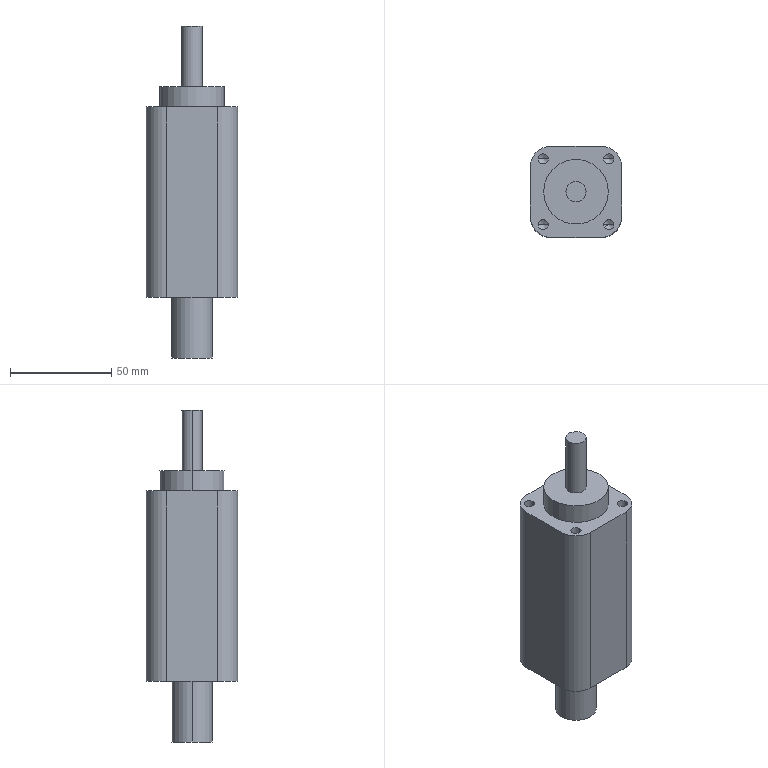Part | 1 solid | 35 faces | box 45 x 45 x 164 mm | volume 200887 mm3 | cylinder 18 | plane 9 | cone 8 | commonest cylinder face diameters 5 x8 20 x6 10 x2 32 x2
STEP:
#1=CARTESIAN_POINT('',(-10.,0.,-30.));
#2=VERTEX_POINT('',#1);
#3=CARTESIAN_POINT('',(10.,0.,-30.));
#4=VERTEX_POINT('',#3);
#5=CARTESIAN_POINT('',(0.,0.,-30.));
#6=DIRECTION('',(0.,0.,-1.));
#7=DIRECTION('',(-1.,0.,0.));
#8=AXIS2_PLACEMENT_3D('',#5,#6,#7);
#9=CIRCLE('',#8,10.);
#10=EDGE_CURVE('',#2,#4,#9,.T.);
#11=ORIENTED_EDGE('',*,*,#10,.F.);
#12=CARTESIAN_POINT('',(-10.,0.,0.));
#13=VERTEX_POINT('',#12);
#14=CARTESIAN_POINT('',(-10.,0.,-30.));
#15=DIRECTION('',(0.,0.,1.));
#16=VECTOR('',#15,1000.);
#17=LINE('',#14,#16);
#18=EDGE_CURVE('',#2,#13,#17,.T.);
#19=ORIENTED_EDGE('',*,*,#18,.T.);
#20=CARTESIAN_POINT('',(10.,0.,0.));
#21=VERTEX_POINT('',#20);
#22=CARTESIAN_POINT('',(0.,0.,0.));
#23=DIRECTION('',(0.,0.,-1.));
#24=DIRECTION('',(-1.,0.,0.));
#25=AXIS2_PLACEMENT_3D('',#22,#23,#24);
#26=CIRCLE('',#25,10.);
#27=EDGE_CURVE('',#13,#21,#26,.T.);
#28=ORIENTED_EDGE('',*,*,#27,.T.);
#29=CARTESIAN_POINT('',(10.,0.,-30.));
#30=DIRECTION('',(0.,0.,1.));
#31=VECTOR('',#30,1000.);
#32=LINE('',#29,#31);
#33=EDGE_CURVE('',#4,#21,#32,.T.);
#34=ORIENTED_EDGE('',*,*,#33,.F.);
#35=EDGE_LOOP('',(#11,#19,#28,#34));
#36=FACE_OUTER_BOUND('',#35,.T.);
#37=CARTESIAN_POINT('',(0.,0.,-30.));
#38=DIRECTION('',(0.,0.,1.));
#39=DIRECTION('',(1.,0.,0.));
#40=AXIS2_PLACEMENT_3D('',#37,#38,#39);
#41=CYLINDRICAL_SURFACE('',#40,10.);
#42=ADVANCED_FACE('',(#36),#41,.T.);
#43=CARTESIAN_POINT('',(5.,0.,134.));
#44=VERTEX_POINT('',#43);
#45=CARTESIAN_POINT('',(-5.,0.,134.));
#46=VERTEX_POINT('',#45);
#47=CARTESIAN_POINT('',(0.,0.,134.));
#48=DIRECTION('',(0.,0.,1.));
#49=DIRECTION('',(1.,0.,0.));
#50=AXIS2_PLACEMENT_3D('',#47,#48,#49);
#51=CIRCLE('',#50,5.);
#52=EDGE_CURVE('',#44,#46,#51,.T.);
#53=ORIENTED_EDGE('',*,*,#52,.F.);
#54=CARTESIAN_POINT('',(5.,0.,104.));
#55=VERTEX_POINT('',#54);
#56=CARTESIAN_POINT('',(5.,0.,134.));
#57=DIRECTION('',(0.,0.,-1.));
#58=VECTOR('',#57,1000.);
#59=LINE('',#56,#58);
#60=EDGE_CURVE('',#44,#55,#59,.T.);
#61=ORIENTED_EDGE('',*,*,#60,.T.);
#62=CARTESIAN_POINT('',(-5.,0.,104.));
#63=VERTEX_POINT('',#62);
#64=CARTESIAN_POINT('',(0.,0.,104.));
#65=DIRECTION('',(0.,0.,1.));
#66=DIRECTION('',(1.,0.,0.));
#67=AXIS2_PLACEMENT_3D('',#64,#65,#66);
#68=CIRCLE('',#67,5.);
#69=EDGE_CURVE('',#55,#63,#68,.T.);
#70=ORIENTED_EDGE('',*,*,#69,.T.);
#71=CARTESIAN_POINT('',(-5.,0.,134.));
#72=DIRECTION('',(0.,0.,-1.));
#73=VECTOR('',#72,1000.);
#74=LINE('',#71,#73);
#75=EDGE_CURVE('',#46,#63,#74,.T.);
#76=ORIENTED_EDGE('',*,*,#75,.F.);
#77=EDGE_LOOP('',(#53,#61,#70,#76));
#78=FACE_OUTER_BOUND('',#77,.T.);
#79=CARTESIAN_POINT('',(0.,0.,134.));
#80=DIRECTION('',(0.,0.,-1.));
#81=DIRECTION('',(-1.,0.,0.));
#82=AXIS2_PLACEMENT_3D('',#79,#80,#81);
#83=CYLINDRICAL_SURFACE('',#82,5.);
#84=ADVANCED_FACE('',(#78),#83,.T.);
#85=CARTESIAN_POINT('',(16.,0.,104.));
#86=VERTEX_POINT('',#85);
#87=CARTESIAN_POINT('',(-16.,0.,104.));
#88=VERTEX_POINT('',#87);
#89=CARTESIAN_POINT('',(0.,0.,104.));
#90=DIRECTION('',(0.,0.,1.));
#91=DIRECTION('',(1.,0.,0.));
#92=AXIS2_PLACEMENT_3D('',#89,#90,#91);
#93=CIRCLE('',#92,16.);
#94=EDGE_CURVE('',#86,#88,#93,.T.);
#95=ORIENTED_EDGE('',*,*,#94,.F.);
#96=CARTESIAN_POINT('',(16.,0.,94.));
#97=VERTEX_POINT('',#96);
#98=CARTESIAN_POINT('',(16.,0.,104.));
#99=DIRECTION('',(0.,0.,-1.));
#100=VECTOR('',#99,1000.);
#101=LINE('',#98,#100);
#102=EDGE_CURVE('',#86,#97,#101,.T.);
#103=ORIENTED_EDGE('',*,*,#102,.T.);
#104=CARTESIAN_POINT('',(-16.,0.,94.));
#105=VERTEX_POINT('',#104);
#106=CARTESIAN_POINT('',(0.,0.,94.));
#107=DIRECTION('',(0.,0.,1.));
#108=DIRECTION('',(-1.,0.,0.));
#109=AXIS2_PLACEMENT_3D('',#106,#107,#108);
#110=CIRCLE('',#109,16.);
#111=EDGE_CURVE('',#97,#105,#110,.T.);
#112=ORIENTED_EDGE('',*,*,#111,.T.);
#113=CARTESIAN_POINT('',(-16.,0.,104.));
#114=DIRECTION('',(0.,0.,-1.));
#115=VECTOR('',#114,1000.);
#116=LINE('',#113,#115);
#117=EDGE_CURVE('',#88,#105,#116,.T.);
#118=ORIENTED_EDGE('',*,*,#117,.F.);
#119=EDGE_LOOP('',(#95,#103,#112,#118));
#120=FACE_OUTER_BOUND('',#119,.T.);
#121=CARTESIAN_POINT('',(0.,0.,104.));
#122=DIRECTION('',(0.,0.,-1.));
#123=DIRECTION('',(-1.,0.,0.));
#124=AXIS2_PLACEMENT_3D('',#121,#122,#123);
#125=CYLINDRICAL_SURFACE('',#124,16.);
#126=ADVANCED_FACE('',(#120),#125,.T.);
#127=CARTESIAN_POINT('',(-18.75,16.25,79.));
#128=VERTEX_POINT('',#127);
#129=CARTESIAN_POINT('',(-13.75,16.25,79.));
#130=VERTEX_POINT('',#129);
#131=CARTESIAN_POINT('',(-16.25,16.25,79.));
#132=DIRECTION('',(0.,0.,1.));
#133=DIRECTION('',(1.,0.,0.));
#134=AXIS2_PLACEMENT_3D('',#131,#132,#133);
#135=CIRCLE('',#134,2.5);
#136=EDGE_CURVE('',#128,#130,#135,.T.);
#137=ORIENTED_EDGE('',*,*,#136,.F.);
#138=CARTESIAN_POINT('',(-18.75,16.25,94.));
#139=VERTEX_POINT('',#138);
#140=CARTESIAN_POINT('',(-18.75,16.25,94.));
#141=DIRECTION('',(0.,0.,1.));
#142=VECTOR('',#141,1000.);
#143=LINE('',#140,#142);
#144=EDGE_CURVE('',#128,#139,#143,.T.);
#145=ORIENTED_EDGE('',*,*,#144,.T.);
#146=CARTESIAN_POINT('',(-13.75,16.25,94.));
#147=VERTEX_POINT('',#146);
#148=CARTESIAN_POINT('',(-16.25,16.25,94.));
#149=DIRECTION('',(0.,0.,1.));
#150=DIRECTION('',(1.,0.,0.));
#151=AXIS2_PLACEMENT_3D('',#148,#149,#150);
#152=CIRCLE('',#151,2.5);
#153=EDGE_CURVE('',#139,#147,#152,.T.);
#154=ORIENTED_EDGE('',*,*,#153,.T.);
#155=CARTESIAN_POINT('',(-13.75,16.25,94.));
#156=DIRECTION('',(0.,0.,1.));
#157=VECTOR('',#156,1000.);
#158=LINE('',#155,#157);
#159=EDGE_CURVE('',#130,#147,#158,.T.);
#160=ORIENTED_EDGE('',*,*,#159,.F.);
#161=EDGE_LOOP('',(#137,#145,#154,#160));
#162=FACE_OUTER_BOUND('',#161,.T.);
#163=CARTESIAN_POINT('',(-16.25,16.25,94.));
#164=DIRECTION('',(0.,0.,1.));
#165=DIRECTION('',(1.,0.,0.));
#166=AXIS2_PLACEMENT_3D('',#163,#164,#165);
#167=CYLINDRICAL_SURFACE('',#166,2.5);
#168=ADVANCED_FACE('',(#162),#167,.F.);
#169=CARTESIAN_POINT('',(-16.25,16.25,77.498));
#170=VERTEX_POINT('',#169);
#171=CARTESIAN_POINT('',(-13.75,16.25,79.));
#172=DIRECTION('',(0.8572,0.,0.515));
#173=VECTOR('',#172,1000.);
#174=LINE('',#171,#173);
#175=EDGE_CURVE('',#170,#130,#174,.T.);
#176=ORIENTED_EDGE('',*,*,#175,.F.);
#177=CARTESIAN_POINT('',(-18.75,16.25,79.));
#178=DIRECTION('',(-0.8572,0.,0.515));
#179=VECTOR('',#178,1000.);
#180=LINE('',#177,#179);
#181=EDGE_CURVE('',#170,#128,#180,.T.);
#182=ORIENTED_EDGE('',*,*,#181,.T.);
#183=ORIENTED_EDGE('',*,*,#136,.T.);
#184=EDGE_LOOP('',(#176,#182,#183));
#185=FACE_OUTER_BOUND('',#184,.T.);
#186=CARTESIAN_POINT('',(-16.25,16.25,79.));
#187=DIRECTION('',(0.,0.,1.));
#188=DIRECTION('',(1.,0.,0.));
#189=AXIS2_PLACEMENT_3D('',#186,#187,#188);
#190=CONICAL_SURFACE('',#189,2.5,1.03);
#191=ADVANCED_FACE('',(#185),#190,.F.);
#192=CARTESIAN_POINT('',(13.75,16.25,79.));
#193=VERTEX_POINT('',#192);
#194=CARTESIAN_POINT('',(18.75,16.25,79.));
#195=VERTEX_POINT('',#194);
#196=CARTESIAN_POINT('',(16.25,16.25,79.));
#197=DIRECTION('',(0.,0.,1.));
#198=DIRECTION('',(1.,0.,0.));
#199=AXIS2_PLACEMENT_3D('',#196,#197,#198);
#200=CIRCLE('',#199,2.5);
#201=EDGE_CURVE('',#193,#195,#200,.T.);
#202=ORIENTED_EDGE('',*,*,#201,.F.);
#203=CARTESIAN_POINT('',(13.75,16.25,94.));
#204=VERTEX_POINT('',#203);
#205=CARTESIAN_POINT('',(13.75,16.25,94.));
#206=DIRECTION('',(0.,0.,1.));
#207=VECTOR('',#206,1000.);
#208=LINE('',#205,#207);
#209=EDGE_CURVE('',#193,#204,#208,.T.);
#210=ORIENTED_EDGE('',*,*,#209,.T.);
#211=CARTESIAN_POINT('',(18.75,16.25,94.));
#212=VERTEX_POINT('',#211);
#213=CARTESIAN_POINT('',(16.25,16.25,94.));
#214=DIRECTION('',(0.,0.,1.));
#215=DIRECTION('',(1.,0.,0.));
#216=AXIS2_PLACEMENT_3D('',#213,#214,#215);
#217=CIRCLE('',#216,2.5);
#218=EDGE_CURVE('',#204,#212,#217,.T.);
#219=ORIENTED_EDGE('',*,*,#218,.T.);
#220=CARTESIAN_POINT('',(18.75,16.25,94.));
#221=DIRECTION('',(0.,0.,1.));
#222=VECTOR('',#221,1000.);
#223=LINE('',#220,#222);
#224=EDGE_CURVE('',#195,#212,#223,.T.);
#225=ORIENTED_EDGE('',*,*,#224,.F.);
#226=EDGE_LOOP('',(#202,#210,#219,#225));
#227=FACE_OUTER_BOUND('',#226,.T.);
#228=CARTESIAN_POINT('',(16.25,16.25,94.));
#229=DIRECTION('',(0.,0.,1.));
#230=DIRECTION('',(1.,0.,0.));
#231=AXIS2_PLACEMENT_3D('',#228,#229,#230);
#232=CYLINDRICAL_SURFACE('',#231,2.5);
#233=ADVANCED_FACE('',(#227),#232,.F.);
#234=CARTESIAN_POINT('',(16.25,16.25,77.498));
#235=VERTEX_POINT('',#234);
#236=CARTESIAN_POINT('',(18.75,16.25,79.));
#237=DIRECTION('',(0.8572,0.,0.515));
#238=VECTOR('',#237,1000.);
#239=LINE('',#236,#238);
#240=EDGE_CURVE('',#235,#195,#239,.T.);
#241=ORIENTED_EDGE('',*,*,#240,.F.);
#242=CARTESIAN_POINT('',(13.75,16.25,79.));
#243=DIRECTION('',(-0.8572,0.,0.515));
#244=VECTOR('',#243,1000.);
#245=LINE('',#242,#244);
#246=EDGE_CURVE('',#235,#193,#245,.T.);
#247=ORIENTED_EDGE('',*,*,#246,.T.);
#248=ORIENTED_EDGE('',*,*,#201,.T.);
#249=EDGE_LOOP('',(#241,#247,#248));
#250=FACE_OUTER_BOUND('',#249,.T.);
#251=CARTESIAN_POINT('',(16.25,16.25,79.));
#252=DIRECTION('',(0.,0.,1.));
#253=DIRECTION('',(1.,0.,0.));
#254=AXIS2_PLACEMENT_3D('',#251,#252,#253);
#255=CONICAL_SURFACE('',#254,2.5,1.03);
#256=ADVANCED_FACE('',(#250),#255,.F.);
#257=CARTESIAN_POINT('',(-18.75,-16.25,79.));
#258=VERTEX_POINT('',#257);
#259=CARTESIAN_POINT('',(-13.75,-16.25,79.));
#260=VERTEX_POINT('',#259);
#261=CARTESIAN_POINT('',(-16.25,-16.25,79.));
#262=DIRECTION('',(0.,0.,1.));
#263=DIRECTION('',(1.,0.,0.));
#264=AXIS2_PLACEMENT_3D('',#261,#262,#263);
#265=CIRCLE('',#264,2.5);
#266=EDGE_CURVE('',#258,#260,#265,.T.);
#267=ORIENTED_EDGE('',*,*,#266,.F.);
#268=CARTESIAN_POINT('',(-18.75,-16.25,94.));
#269=VERTEX_POINT('',#268);
#270=CARTESIAN_POINT('',(-18.75,-16.25,94.));
#271=DIRECTION('',(0.,0.,1.));
#272=VECTOR('',#271,1000.);
#273=LINE('',#270,#272);
#274=EDGE_CURVE('',#258,#269,#273,.T.);
#275=ORIENTED_EDGE('',*,*,#274,.T.);
#276=CARTESIAN_POINT('',(-13.75,-16.25,94.));
#277=VERTEX_POINT('',#276);
#278=CARTESIAN_POINT('',(-16.25,-16.25,94.));
#279=DIRECTION('',(0.,0.,1.));
#280=DIRECTION('',(1.,0.,0.));
#281=AXIS2_PLACEMENT_3D('',#278,#279,#280);
#282=CIRCLE('',#281,2.5);
#283=EDGE_CURVE('',#269,#277,#282,.T.);
#284=ORIENTED_EDGE('',*,*,#283,.T.);
#285=CARTESIAN_POINT('',(-13.75,-16.25,94.));
#286=DIRECTION('',(0.,0.,1.));
#287=VECTOR('',#286,1000.);
#288=LINE('',#285,#287);
#289=EDGE_CURVE('',#260,#277,#288,.T.);
#290=ORIENTED_EDGE('',*,*,#289,.F.);
#291=EDGE_LOOP('',(#267,#275,#284,#290));
#292=FACE_OUTER_BOUND('',#291,.T.);
#293=CARTESIAN_POINT('',(-16.25,-16.25,94.));
#294=DIRECTION('',(0.,0.,1.));
#295=DIRECTION('',(1.,0.,0.));
#296=AXIS2_PLACEMENT_3D('',#293,#294,#295);
#297=CYLINDRICAL_SURFACE('',#296,2.5);
#298=ADVANCED_FACE('',(#292),#297,.F.);
#299=CARTESIAN_POINT('',(-16.25,-16.25,77.498));
#300=VERTEX_POINT('',#299);
#301=CARTESIAN_POINT('',(-13.75,-16.25,79.));
#302=DIRECTION('',(0.8572,0.,0.515));
#303=VECTOR('',#302,1000.);
#304=LINE('',#301,#303);
#305=EDGE_CURVE('',#300,#260,#304,.T.);
#306=ORIENTED_EDGE('',*,*,#305,.F.);
#307=CARTESIAN_POINT('',(-18.75,-16.25,79.));
#308=DIRECTION('',(-0.8572,0.,0.515));
#309=VECTOR('',#308,1000.);
#310=LINE('',#307,#309);
#311=EDGE_CURVE('',#300,#258,#310,.T.);
#312=ORIENTED_EDGE('',*,*,#311,.T.);
#313=ORIENTED_EDGE('',*,*,#266,.T.);
#314=EDGE_LOOP('',(#306,#312,#313));
#315=FACE_OUTER_BOUND('',#314,.T.);
#316=CARTESIAN_POINT('',(-16.25,-16.25,79.));
#317=DIRECTION('',(0.,0.,1.));
#318=DIRECTION('',(1.,0.,0.));
#319=AXIS2_PLACEMENT_3D('',#316,#317,#318);
#320=CONICAL_SURFACE('',#319,2.5,1.03);
#321=ADVANCED_FACE('',(#315),#320,.F.);
#322=CARTESIAN_POINT('',(13.75,-16.25,79.));
#323=VERTEX_POINT('',#322);
#324=CARTESIAN_POINT('',(18.75,-16.25,79.));
#325=VERTEX_POINT('',#324);
#326=CARTESIAN_POINT('',(16.25,-16.25,79.));
#327=DIRECTION('',(0.,0.,1.));
#328=DIRECTION('',(1.,0.,0.));
#329=AXIS2_PLACEMENT_3D('',#326,#327,#328);
#330=CIRCLE('',#329,2.5);
#331=EDGE_CURVE('',#323,#325,#330,.T.);
#332=ORIENTED_EDGE('',*,*,#331,.F.);
#333=CARTESIAN_POINT('',(13.75,-16.25,94.));
#334=VERTEX_POINT('',#333);
#335=CARTESIAN_POINT('',(13.75,-16.25,94.));
#336=DIRECTION('',(0.,0.,1.));
#337=VECTOR('',#336,1000.);
#338=LINE('',#335,#337);
#339=EDGE_CURVE('',#323,#334,#338,.T.);
#340=ORIENTED_EDGE('',*,*,#339,.T.);
#341=CARTESIAN_POINT('',(18.75,-16.25,94.));
#342=VERTEX_POINT('',#341);
#343=CARTESIAN_POINT('',(16.25,-16.25,94.));
#344=DIRECTION('',(0.,0.,1.));
#345=DIRECTION('',(1.,0.,0.));
#346=AXIS2_PLACEMENT_3D('',#343,#344,#345);
#347=CIRCLE('',#346,2.5);
#348=EDGE_CURVE('',#334,#342,#347,.T.);
#349=ORIENTED_EDGE('',*,*,#348,.T.);
#350=CARTESIAN_POINT('',(18.75,-16.25,94.));
#351=DIRECTION('',(0.,0.,1.));
#352=VECTOR('',#351,1000.);
#353=LINE('',#350,#352);
#354=EDGE_CURVE('',#325,#342,#353,.T.);
#355=ORIENTED_EDGE('',*,*,#354,.F.);
#356=EDGE_LOOP('',(#332,#340,#349,#355));
#357=FACE_OUTER_BOUND('',#356,.T.);
#358=CARTESIAN_POINT('',(16.25,-16.25,94.));
#359=DIRECTION('',(0.,0.,1.));
#360=DIRECTION('',(1.,0.,0.));
#361=AXIS2_PLACEMENT_3D('',#358,#359,#360);
#362=CYLINDRICAL_SURFACE('',#361,2.5);
#363=ADVANCED_FACE('',(#357),#362,.F.);
#364=CARTESIAN_POINT('',(16.25,-16.25,77.498));
#365=VERTEX_POINT('',#364);
#366=CARTESIAN_POINT('',(18.75,-16.25,79.));
#367=DIRECTION('',(0.8572,0.,0.515));
#368=VECTOR('',#367,1000.);
#369=LINE('',#366,#368);
#370=EDGE_CURVE('',#365,#325,#369,.T.);
#371=ORIENTED_EDGE('',*,*,#370,.F.);
#372=CARTESIAN_POINT('',(13.75,-16.25,79.));
#373=DIRECTION('',(-0.8572,0.,0.515));
#374=VECTOR('',#373,1000.);
#375=LINE('',#372,#374);
#376=EDGE_CURVE('',#365,#323,#375,.T.);
#377=ORIENTED_EDGE('',*,*,#376,.T.);
#378=ORIENTED_EDGE('',*,*,#331,.T.);
#379=EDGE_LOOP('',(#371,#377,#378));
#380=FACE_OUTER_BOUND('',#379,.T.);
#381=CARTESIAN_POINT('',(16.25,-16.25,79.));
#382=DIRECTION('',(0.,0.,1.));
#383=DIRECTION('',(1.,0.,0.));
#384=AXIS2_PLACEMENT_3D('',#381,#382,#383);
#385=CONICAL_SURFACE('',#384,2.5,1.03);
#386=ADVANCED_FACE('',(#380),#385,.F.);
#387=CARTESIAN_POINT('',(-12.5,-22.5,0.));
#388=VERTEX_POINT('',#387);
#389=CARTESIAN_POINT('',(12.5,-22.5,0.));
#390=VERTEX_POINT('',#389);
#391=CARTESIAN_POINT('',(-22.5,-22.5,0.));
#392=DIRECTION('',(1.,0.,0.));
#393=VECTOR('',#392,1000.);
#394=LINE('',#391,#393);
#395=EDGE_CURVE('',#388,#390,#394,.T.);
#396=ORIENTED_EDGE('',*,*,#395,.F.);
#397=CARTESIAN_POINT('',(-22.5,-12.5,0.));
#398=VERTEX_POINT('',#397);
#399=CARTESIAN_POINT('',(-12.5,-12.5,0.));
#400=DIRECTION('',(0.,0.,-1.));
#401=DIRECTION('',(-1.,0.,0.));
#402=AXIS2_PLACEMENT_3D('',#399,#400,#401);
#403=CIRCLE('',#402,10.);
#404=EDGE_CURVE('',#388,#398,#403,.T.);
#405=ORIENTED_EDGE('',*,*,#404,.T.);
#406=CARTESIAN_POINT('',(-22.5,12.5,0.));
#407=VERTEX_POINT('',#406);
#408=CARTESIAN_POINT('',(-22.5,-22.5,0.));
#409=DIRECTION('',(0.,-1.,0.));
#410=VECTOR('',#409,1000.);
#411=LINE('',#408,#410);
#412=EDGE_CURVE('',#407,#398,#411,.T.);
#413=ORIENTED_EDGE('',*,*,#412,.F.);
#414=CARTESIAN_POINT('',(-12.5,22.5,0.));
#415=VERTEX_POINT('',#414);
#416=CARTESIAN_POINT('',(-12.5,12.5,0.));
#417=DIRECTION('',(0.,0.,-1.));
#418=DIRECTION('',(-1.,0.,0.));
#419=AXIS2_PLACEMENT_3D('',#416,#417,#418);
#420=CIRCLE('',#419,10.);
#421=EDGE_CURVE('',#407,#415,#420,.T.);
#422=ORIENTED_EDGE('',*,*,#421,.T.);
#423=CARTESIAN_POINT('',(12.5,22.5,0.));
#424=VERTEX_POINT('',#423);
#425=CARTESIAN_POINT('',(-22.5,22.5,0.));
#426=DIRECTION('',(-1.,0.,0.));
#427=VECTOR('',#426,1000.);
#428=LINE('',#425,#427);
#429=EDGE_CURVE('',#424,#415,#428,.T.);
#430=ORIENTED_EDGE('',*,*,#429,.F.);
#431=CARTESIAN_POINT('',(22.5,12.5,0.));
#432=VERTEX_POINT('',#431);
#433=CARTESIAN_POINT('',(12.5,12.5,0.));
#434=DIRECTION('',(0.,0.,-1.));
#435=DIRECTION('',(-1.,0.,0.));
#436=AXIS2_PLACEMENT_3D('',#433,#434,#435);
#437=CIRCLE('',#436,10.);
#438=EDGE_CURVE('',#424,#432,#437,.T.);
#439=ORIENTED_EDGE('',*,*,#438,.T.);
#440=CARTESIAN_POINT('',(22.5,-12.5,0.));
#441=VERTEX_POINT('',#440);
#442=CARTESIAN_POINT('',(22.5,-22.5,0.));
#443=DIRECTION('',(0.,1.,0.));
#444=VECTOR('',#443,1000.);
#445=LINE('',#442,#444);
#446=EDGE_CURVE('',#441,#432,#445,.T.);
#447=ORIENTED_EDGE('',*,*,#446,.F.);
#448=CARTESIAN_POINT('',(12.5,-12.5,0.));
#449=DIRECTION('',(0.,0.,-1.));
#450=DIRECTION('',(-1.,0.,0.));
#451=AXIS2_PLACEMENT_3D('',#448,#449,#450);
#452=CIRCLE('',#451,10.);
#453=EDGE_CURVE('',#441,#390,#452,.T.);
#454=ORIENTED_EDGE('',*,*,#453,.T.);
#455=EDGE_LOOP('',(#396,#405,#413,#422,#430,#439,#447,#454));
#456=FACE_OUTER_BOUND('',#455,.T.);
#457=CARTESIAN_POINT('',(0.,0.,0.));
#458=DIRECTION('',(0.,0.,-1.));
#459=DIRECTION('',(-1.,0.,0.));
#460=AXIS2_PLACEMENT_3D('',#457,#458,#459);
#461=CIRCLE('',#460,10.);
#462=EDGE_CURVE('',#21,#13,#461,.T.);
#463=ORIENTED_EDGE('',*,*,#462,.F.);
#464=ORIENTED_EDGE('',*,*,#27,.F.);
#465=EDGE_LOOP('',(#463,#464));
#466=FACE_BOUND('',#465,.T.);
#467=CARTESIAN_POINT('',(0.,0.,0.));
#468=DIRECTION('',(0.,0.,-1.));
#469=DIRECTION('',(-1.,0.,0.));
#470=AXIS2_PLACEMENT_3D('',#467,#468,#469);
#471=PLANE('',#470);
#472=ADVANCED_FACE('',(#456,#466),#471,.T.);
#473=CARTESIAN_POINT('',(0.,0.,104.));
#474=DIRECTION('',(0.,0.,1.));
#475=DIRECTION('',(1.,0.,0.));
#476=AXIS2_PLACEMENT_3D('',#473,#474,#475);
#477=CIRCLE('',#476,16.);
#478=EDGE_CURVE('',#88,#86,#477,.T.);
#479=ORIENTED_EDGE('',*,*,#478,.T.);
#480=ORIENTED_EDGE('',*,*,#94,.T.);
#481=EDGE_LOOP('',(#479,#480));
#482=FACE_OUTER_BOUND('',#481,.T.);
#483=CARTESIAN_POINT('',(0.,0.,104.));
#484=DIRECTION('',(0.,0.,1.));
#485=DIRECTION('',(1.,0.,0.));
#486=AXIS2_PLACEMENT_3D('',#483,#484,#485);
#487=CIRCLE('',#486,5.);
#488=EDGE_CURVE('',#63,#55,#487,.T.);
#489=ORIENTED_EDGE('',*,*,#488,.F.);
#490=ORIENTED_EDGE('',*,*,#69,.F.);
#491=EDGE_LOOP('',(#489,#490));
#492=FACE_BOUND('',#491,.T.);
#493=CARTESIAN_POINT('',(0.,0.,104.));
#494=DIRECTION('',(0.,0.,1.));
#495=DIRECTION('',(1.,0.,0.));
#496=AXIS2_PLACEMENT_3D('',#493,#494,#495);
#497=PLANE('',#496);
#498=ADVANCED_FACE('',(#482,#492),#497,.T.);
#499=CARTESIAN_POINT('',(-22.5,12.5,94.));
#500=VERTEX_POINT('',#499);
#501=CARTESIAN_POINT('',(-22.5,-12.5,94.));
#502=VERTEX_POINT('',#501);
#503=CARTESIAN_POINT('',(-22.5,-22.5,94.));
#504=DIRECTION('',(0.,-1.,0.));
#505=VECTOR('',#504,1000.);
#506=LINE('',#503,#505);
#507=EDGE_CURVE('',#500,#502,#506,.T.);
#508=ORIENTED_EDGE('',*,*,#507,.T.);
#509=CARTESIAN_POINT('',(-12.5,-22.5,94.));
#510=VERTEX_POINT('',#509);
#511=CARTESIAN_POINT('',(-12.5,-12.5,94.));
#512=DIRECTION('',(0.,0.,1.));
#513=DIRECTION('',(-1.,0.,0.));
#514=AXIS2_PLACEMENT_3D('',#511,#512,#513);
#515=CIRCLE('',#514,10.);
#516=EDGE_CURVE('',#502,#510,#515,.T.);
#517=ORIENTED_EDGE('',*,*,#516,.T.);
#518=CARTESIAN_POINT('',(12.5,-22.5,94.));
#519=VERTEX_POINT('',#518);
#520=CARTESIAN_POINT('',(-22.5,-22.5,94.));
#521=DIRECTION('',(1.,0.,0.));
#522=VECTOR('',#521,1000.);
#523=LINE('',#520,#522);
#524=EDGE_CURVE('',#510,#519,#523,.T.);
#525=ORIENTED_EDGE('',*,*,#524,.T.);
#526=CARTESIAN_POINT('',(22.5,-12.5,94.));
#527=VERTEX_POINT('',#526);
#528=CARTESIAN_POINT('',(12.5,-12.5,94.));
#529=DIRECTION('',(0.,0.,1.));
#530=DIRECTION('',(-1.,0.,0.));
#531=AXIS2_PLACEMENT_3D('',#528,#529,#530);
#532=CIRCLE('',#531,10.);
#533=EDGE_CURVE('',#519,#527,#532,.T.);
#534=ORIENTED_EDGE('',*,*,#533,.T.);
#535=CARTESIAN_POINT('',(22.5,12.5,94.));
#536=VERTEX_POINT('',#535);
#537=CARTESIAN_POINT('',(22.5,-22.5,94.));
#538=DIRECTION('',(0.,1.,0.));
#539=VECTOR('',#538,1000.);
#540=LINE('',#537,#539);
#541=EDGE_CURVE('',#527,#536,#540,.T.);
#542=ORIENTED_EDGE('',*,*,#541,.T.);
#543=CARTESIAN_POINT('',(12.5,22.5,94.));
#544=VERTEX_POINT('',#543);
#545=CARTESIAN_POINT('',(12.5,12.5,94.));
#546=DIRECTION('',(0.,0.,1.));
#547=DIRECTION('',(-1.,0.,0.));
#548=AXIS2_PLACEMENT_3D('',#545,#546,#547);
#549=CIRCLE('',#548,10.);
#550=EDGE_CURVE('',#536,#544,#549,.T.);
#551=ORIENTED_EDGE('',*,*,#550,.T.);
#552=CARTESIAN_POINT('',(-12.5,22.5,94.));
#553=VERTEX_POINT('',#552);
#554=CARTESIAN_POINT('',(-22.5,22.5,94.));
#555=DIRECTION('',(-1.,0.,0.));
#556=VECTOR('',#555,1000.);
#557=LINE('',#554,#556);
#558=EDGE_CURVE('',#544,#553,#557,.T.);
#559=ORIENTED_EDGE('',*,*,#558,.T.);
#560=CARTESIAN_POINT('',(-12.5,12.5,94.));
#561=DIRECTION('',(0.,0.,1.));
#562=DIRECTION('',(-1.,0.,0.));
#563=AXIS2_PLACEMENT_3D('',#560,#561,#562);
#564=CIRCLE('',#563,10.);
#565=EDGE_CURVE('',#553,#500,#564,.T.);
#566=ORIENTED_EDGE('',*,*,#565,.T.);
#567=EDGE_LOOP('',(#508,#517,#525,#534,#542,#551,#559,#566));
#568=FACE_OUTER_BOUND('',#567,.T.);
#569=CARTESIAN_POINT('',(16.25,-16.25,94.));
#570=DIRECTION('',(0.,0.,1.));
#571=DIRECTION('',(1.,0.,0.));
#572=AXIS2_PLACEMENT_3D('',#569,#570,#571);
#573=CIRCLE('',#572,2.5);
#574=EDGE_CURVE('',#342,#334,#573,.T.);
#575=ORIENTED_EDGE('',*,*,#574,.F.);
#576=ORIENTED_EDGE('',*,*,#348,.F.);
#577=EDGE_LOOP('',(#575,#576));
#578=FACE_BOUND('',#577,.T.);
#579=CARTESIAN_POINT('',(-16.25,-16.25,94.));
#580=DIRECTION('',(0.,0.,1.));
#581=DIRECTION('',(1.,0.,0.));
#582=AXIS2_PLACEMENT_3D('',#579,#580,#581);
#583=CIRCLE('',#582,2.5);
#584=EDGE_CURVE('',#277,#269,#583,.T.);
#585=ORIENTED_EDGE('',*,*,#584,.F.);
#586=ORIENTED_EDGE('',*,*,#283,.F.);
#587=EDGE_LOOP('',(#585,#586));
#588=FACE_BOUND('',#587,.T.);
#589=CARTESIAN_POINT('',(16.25,16.25,94.));
#590=DIRECTION('',(0.,0.,1.));
#591=DIRECTION('',(1.,0.,0.));
#592=AXIS2_PLACEMENT_3D('',#589,#590,#591);
#593=CIRCLE('',#592,2.5);
#594=EDGE_CURVE('',#212,#204,#593,.T.);
#595=ORIENTED_EDGE('',*,*,#594,.F.);
#596=ORIENTED_EDGE('',*,*,#218,.F.);
#597=EDGE_LOOP('',(#595,#596));
#598=FACE_BOUND('',#597,.T.);
#599=CARTESIAN_POINT('',(-16.25,16.25,94.));
#600=DIRECTION('',(0.,0.,1.));
#601=DIRECTION('',(1.,0.,0.));
#602=AXIS2_PLACEMENT_3D('',#599,#600,#601);
#603=CIRCLE('',#602,2.5);
#604=EDGE_CURVE('',#147,#139,#603,.T.);
#605=ORIENTED_EDGE('',*,*,#604,.F.);
#606=ORIENTED_EDGE('',*,*,#153,.F.);
#607=EDGE_LOOP('',(#605,#606));
#608=FACE_BOUND('',#607,.T.);
#609=CARTESIAN_POINT('',(0.,0.,94.));
#610=DIRECTION('',(0.,0.,1.));
#611=DIRECTION('',(-1.,0.,0.));
#612=AXIS2_PLACEMENT_3D('',#609,#610,#611);
#613=CIRCLE('',#612,16.);
#614=EDGE_CURVE('',#105,#97,#613,.T.);
#615=ORIENTED_EDGE('',*,*,#614,.F.);
#616=ORIENTED_EDGE('',*,*,#111,.F.);
#617=EDGE_LOOP('',(#615,#616));
#618=FACE_BOUND('',#617,.T.);
#619=CARTESIAN_POINT('',(0.,0.,94.));
#620=DIRECTION('',(0.,0.,-1.));
#621=DIRECTION('',(-1.,0.,0.));
#622=AXIS2_PLACEMENT_3D('',#619,#620,#621);
#623=PLANE('',#622);
#624=ADVANCED_FACE('',(#568,#578,#588,#598,#608,#618),#623,.F.);
#625=ORIENTED_EDGE('',*,*,#541,.F.);
#626=CARTESIAN_POINT('',(22.5,-12.5,94.));
#627=DIRECTION('',(0.,0.,-1.));
#628=VECTOR('',#627,1000.);
#629=LINE('',#626,#628);
#630=EDGE_CURVE('',#527,#441,#629,.T.);
#631=ORIENTED_EDGE('',*,*,#630,.T.);
#632=ORIENTED_EDGE('',*,*,#446,.T.);
#633=CARTESIAN_POINT('',(22.5,12.5,94.));
#634=DIRECTION('',(0.,0.,1.));
#635=VECTOR('',#634,1000.);
#636=LINE('',#633,#635);
#637=EDGE_CURVE('',#432,#536,#636,.T.);
#638=ORIENTED_EDGE('',*,*,#637,.T.);
#639=EDGE_LOOP('',(#625,#631,#632,#638));
#640=FACE_OUTER_BOUND('',#639,.T.);
#641=CARTESIAN_POINT('',(22.5,-22.5,94.));
#642=DIRECTION('',(-1.,0.,0.));
#643=DIRECTION('',(0.,0.,1.));
#644=AXIS2_PLACEMENT_3D('',#641,#642,#643);
#645=PLANE('',#644);
#646=ADVANCED_FACE('',(#640),#645,.F.);
#647=ORIENTED_EDGE('',*,*,#429,.T.);
#648=CARTESIAN_POINT('',(-12.5,22.5,94.));
#649=DIRECTION('',(0.,0.,1.));
#650=VECTOR('',#649,1000.);
#651=LINE('',#648,#650);
#652=EDGE_CURVE('',#415,#553,#651,.T.);
#653=ORIENTED_EDGE('',*,*,#652,.T.);
#654=ORIENTED_EDGE('',*,*,#558,.F.);
#655=CARTESIAN_POINT('',(12.5,22.5,94.));
#656=DIRECTION('',(0.,0.,-1.));
#657=VECTOR('',#656,1000.);
#658=LINE('',#655,#657);
#659=EDGE_CURVE('',#544,#424,#658,.T.);
#660=ORIENTED_EDGE('',*,*,#659,.T.);
#661=EDGE_LOOP('',(#647,#653,#654,#660));
#662=FACE_OUTER_BOUND('',#661,.T.);
#663=CARTESIAN_POINT('',(-22.5,22.5,94.));
#664=DIRECTION('',(0.,-1.,0.));
#665=DIRECTION('',(0.,0.,-1.));
#666=AXIS2_PLACEMENT_3D('',#663,#664,#665);
#667=PLANE('',#666);
#668=ADVANCED_FACE('',(#662),#667,.F.);
#669=ORIENTED_EDGE('',*,*,#412,.T.);
#670=CARTESIAN_POINT('',(-22.5,-12.5,94.));
#671=DIRECTION('',(0.,0.,1.));
#672=VECTOR('',#671,1000.);
#673=LINE('',#670,#672);
#674=EDGE_CURVE('',#398,#502,#673,.T.);
#675=ORIENTED_EDGE('',*,*,#674,.T.);
#676=ORIENTED_EDGE('',*,*,#507,.F.);
#677=CARTESIAN_POINT('',(-22.5,12.5,94.));
#678=DIRECTION('',(0.,0.,-1.));
#679=VECTOR('',#678,1000.);
#680=LINE('',#677,#679);
#681=EDGE_CURVE('',#500,#407,#680,.T.);
#682=ORIENTED_EDGE('',*,*,#681,.T.);
#683=EDGE_LOOP('',(#669,#675,#676,#682));
#684=FACE_OUTER_BOUND('',#683,.T.);
#685=CARTESIAN_POINT('',(-22.5,-22.5,94.));
#686=DIRECTION('',(1.,0.,0.));
#687=DIRECTION('',(0.,0.,-1.));
#688=AXIS2_PLACEMENT_3D('',#685,#686,#687);
#689=PLANE('',#688);
#690=ADVANCED_FACE('',(#684),#689,.F.);
#691=ORIENTED_EDGE('',*,*,#524,.F.);
#692=CARTESIAN_POINT('',(-12.5,-22.5,94.));
#693=DIRECTION('',(0.,0.,-1.));
#694=VECTOR('',#693,1000.);
#695=LINE('',#692,#694);
#696=EDGE_CURVE('',#510,#388,#695,.T.);
#697=ORIENTED_EDGE('',*,*,#696,.T.);
#698=ORIENTED_EDGE('',*,*,#395,.T.);
#699=CARTESIAN_POINT('',(12.5,-22.5,94.));
#700=DIRECTION('',(0.,0.,1.));
#701=VECTOR('',#700,1000.);
#702=LINE('',#699,#701);
#703=EDGE_CURVE('',#390,#519,#702,.T.);
#704=ORIENTED_EDGE('',*,*,#703,.T.);
#705=EDGE_LOOP('',(#691,#697,#698,#704));
#706=FACE_OUTER_BOUND('',#705,.T.);
#707=CARTESIAN_POINT('',(-22.5,-22.5,94.));
#708=DIRECTION('',(0.,1.,0.));
#709=DIRECTION('',(0.,0.,1.));
#710=AXIS2_PLACEMENT_3D('',#707,#708,#709);
#711=PLANE('',#710);
#712=ADVANCED_FACE('',(#706),#711,.F.);
#713=ORIENTED_EDGE('',*,*,#376,.F.);
#714=ORIENTED_EDGE('',*,*,#370,.T.);
#715=CARTESIAN_POINT('',(16.25,-16.25,79.));
#716=DIRECTION('',(0.,0.,1.));
#717=DIRECTION('',(1.,0.,0.));
#718=AXIS2_PLACEMENT_3D('',#715,#716,#717);
#719=CIRCLE('',#718,2.5);
#720=EDGE_CURVE('',#325,#323,#719,.T.);
#721=ORIENTED_EDGE('',*,*,#720,.T.);
#722=EDGE_LOOP('',(#713,#714,#721));
#723=FACE_OUTER_BOUND('',#722,.T.);
#724=CARTESIAN_POINT('',(16.25,-16.25,79.));
#725=DIRECTION('',(0.,0.,1.));
#726=DIRECTION('',(1.,0.,0.));
#727=AXIS2_PLACEMENT_3D('',#724,#725,#726);
#728=CONICAL_SURFACE('',#727,2.5,1.03);
#729=ADVANCED_FACE('',(#723),#728,.F.);
#730=ORIENTED_EDGE('',*,*,#339,.F.);
#731=ORIENTED_EDGE('',*,*,#720,.F.);
#732=ORIENTED_EDGE('',*,*,#354,.T.);
#733=ORIENTED_EDGE('',*,*,#574,.T.);
#734=EDGE_LOOP('',(#730,#731,#732,#733));
#735=FACE_OUTER_BOUND('',#734,.T.);
#736=CARTESIAN_POINT('',(16.25,-16.25,94.));
#737=DIRECTION('',(0.,0.,1.));
#738=DIRECTION('',(1.,0.,0.));
#739=AXIS2_PLACEMENT_3D('',#736,#737,#738);
#740=CYLINDRICAL_SURFACE('',#739,2.5);
#741=ADVANCED_FACE('',(#735),#740,.F.);
#742=ORIENTED_EDGE('',*,*,#311,.F.);
#743=ORIENTED_EDGE('',*,*,#305,.T.);
#744=CARTESIAN_POINT('',(-16.25,-16.25,79.));
#745=DIRECTION('',(0.,0.,1.));
#746=DIRECTION('',(1.,0.,0.));
#747=AXIS2_PLACEMENT_3D('',#744,#745,#746);
#748=CIRCLE('',#747,2.5);
#749=EDGE_CURVE('',#260,#258,#748,.T.);
#750=ORIENTED_EDGE('',*,*,#749,.T.);
#751=EDGE_LOOP('',(#742,#743,#750));
#752=FACE_OUTER_BOUND('',#751,.T.);
#753=CARTESIAN_POINT('',(-16.25,-16.25,79.));
#754=DIRECTION('',(0.,0.,1.));
#755=DIRECTION('',(1.,0.,0.));
#756=AXIS2_PLACEMENT_3D('',#753,#754,#755);
#757=CONICAL_SURFACE('',#756,2.5,1.03);
#758=ADVANCED_FACE('',(#752),#757,.F.);
#759=ORIENTED_EDGE('',*,*,#274,.F.);
#760=ORIENTED_EDGE('',*,*,#749,.F.);
#761=ORIENTED_EDGE('',*,*,#289,.T.);
#762=ORIENTED_EDGE('',*,*,#584,.T.);
#763=EDGE_LOOP('',(#759,#760,#761,#762));
#764=FACE_OUTER_BOUND('',#763,.T.);
#765=CARTESIAN_POINT('',(-16.25,-16.25,94.));
#766=DIRECTION('',(0.,0.,1.));
#767=DIRECTION('',(1.,0.,0.));
#768=AXIS2_PLACEMENT_3D('',#765,#766,#767);
#769=CYLINDRICAL_SURFACE('',#768,2.5);
#770=ADVANCED_FACE('',(#764),#769,.F.);
#771=ORIENTED_EDGE('',*,*,#246,.F.);
#772=ORIENTED_EDGE('',*,*,#240,.T.);
#773=CARTESIAN_POINT('',(16.25,16.25,79.));
#774=DIRECTION('',(0.,0.,1.));
#775=DIRECTION('',(1.,0.,0.));
#776=AXIS2_PLACEMENT_3D('',#773,#774,#775);
#777=CIRCLE('',#776,2.5);
#778=EDGE_CURVE('',#195,#193,#777,.T.);
#779=ORIENTED_EDGE('',*,*,#778,.T.);
#780=EDGE_LOOP('',(#771,#772,#779));
#781=FACE_OUTER_BOUND('',#780,.T.);
#782=CARTESIAN_POINT('',(16.25,16.25,79.));
#783=DIRECTION('',(0.,0.,1.));
#784=DIRECTION('',(1.,0.,0.));
#785=AXIS2_PLACEMENT_3D('',#782,#783,#784);
#786=CONICAL_SURFACE('',#785,2.5,1.03);
#787=ADVANCED_FACE('',(#781),#786,.F.);
#788=ORIENTED_EDGE('',*,*,#209,.F.);
#789=ORIENTED_EDGE('',*,*,#778,.F.);
#790=ORIENTED_EDGE('',*,*,#224,.T.);
#791=ORIENTED_EDGE('',*,*,#594,.T.);
#792=EDGE_LOOP('',(#788,#789,#790,#791));
#793=FACE_OUTER_BOUND('',#792,.T.);
#794=CARTESIAN_POINT('',(16.25,16.25,94.));
#795=DIRECTION('',(0.,0.,1.));
#796=DIRECTION('',(1.,0.,0.));
#797=AXIS2_PLACEMENT_3D('',#794,#795,#796);
#798=CYLINDRICAL_SURFACE('',#797,2.5);
#799=ADVANCED_FACE('',(#793),#798,.F.);
#800=ORIENTED_EDGE('',*,*,#181,.F.);
#801=ORIENTED_EDGE('',*,*,#175,.T.);
#802=CARTESIAN_POINT('',(-16.25,16.25,79.));
#803=DIRECTION('',(0.,0.,1.));
#804=DIRECTION('',(1.,0.,0.));
#805=AXIS2_PLACEMENT_3D('',#802,#803,#804);
#806=CIRCLE('',#805,2.5);
#807=EDGE_CURVE('',#130,#128,#806,.T.);
#808=ORIENTED_EDGE('',*,*,#807,.T.);
#809=EDGE_LOOP('',(#800,#801,#808));
#810=FACE_OUTER_BOUND('',#809,.T.);
#811=CARTESIAN_POINT('',(-16.25,16.25,79.));
#812=DIRECTION('',(0.,0.,1.));
#813=DIRECTION('',(1.,0.,0.));
#814=AXIS2_PLACEMENT_3D('',#811,#812,#813);
#815=CONICAL_SURFACE('',#814,2.5,1.03);
#816=ADVANCED_FACE('',(#810),#815,.F.);
#817=ORIENTED_EDGE('',*,*,#144,.F.);
#818=ORIENTED_EDGE('',*,*,#807,.F.);
#819=ORIENTED_EDGE('',*,*,#159,.T.);
#820=ORIENTED_EDGE('',*,*,#604,.T.);
#821=EDGE_LOOP('',(#817,#818,#819,#820));
#822=FACE_OUTER_BOUND('',#821,.T.);
#823=CARTESIAN_POINT('',(-16.25,16.25,94.));
#824=DIRECTION('',(0.,0.,1.));
#825=DIRECTION('',(1.,0.,0.));
#826=AXIS2_PLACEMENT_3D('',#823,#824,#825);
#827=CYLINDRICAL_SURFACE('',#826,2.5);
#828=ADVANCED_FACE('',(#822),#827,.F.);
#829=ORIENTED_EDGE('',*,*,#516,.F.);
#830=ORIENTED_EDGE('',*,*,#674,.F.);
#831=ORIENTED_EDGE('',*,*,#404,.F.);
#832=ORIENTED_EDGE('',*,*,#696,.F.);
#833=EDGE_LOOP('',(#829,#830,#831,#832));
#834=FACE_OUTER_BOUND('',#833,.T.);
#835=CARTESIAN_POINT('',(-12.5,-12.5,94.));
#836=DIRECTION('',(0.,0.,-1.));
#837=DIRECTION('',(-1.,0.,0.));
#838=AXIS2_PLACEMENT_3D('',#835,#836,#837);
#839=CYLINDRICAL_SURFACE('',#838,10.);
#840=ADVANCED_FACE('',(#834),#839,.T.);
#841=ORIENTED_EDGE('',*,*,#533,.F.);
#842=ORIENTED_EDGE('',*,*,#703,.F.);
#843=ORIENTED_EDGE('',*,*,#453,.F.);
#844=ORIENTED_EDGE('',*,*,#630,.F.);
#845=EDGE_LOOP('',(#841,#842,#843,#844));
#846=FACE_OUTER_BOUND('',#845,.T.);
#847=CARTESIAN_POINT('',(12.5,-12.5,94.));
#848=DIRECTION('',(0.,0.,-1.));
#849=DIRECTION('',(-1.,0.,0.));
#850=AXIS2_PLACEMENT_3D('',#847,#848,#849);
#851=CYLINDRICAL_SURFACE('',#850,10.);
#852=ADVANCED_FACE('',(#846),#851,.T.);
#853=ORIENTED_EDGE('',*,*,#565,.F.);
#854=ORIENTED_EDGE('',*,*,#652,.F.);
#855=ORIENTED_EDGE('',*,*,#421,.F.);
#856=ORIENTED_EDGE('',*,*,#681,.F.);
#857=EDGE_LOOP('',(#853,#854,#855,#856));
#858=FACE_OUTER_BOUND('',#857,.T.);
#859=CARTESIAN_POINT('',(-12.5,12.5,94.));
#860=DIRECTION('',(0.,0.,-1.));
#861=DIRECTION('',(-1.,0.,0.));
#862=AXIS2_PLACEMENT_3D('',#859,#860,#861);
#863=CYLINDRICAL_SURFACE('',#862,10.);
#864=ADVANCED_FACE('',(#858),#863,.T.);
#865=ORIENTED_EDGE('',*,*,#550,.F.);
#866=ORIENTED_EDGE('',*,*,#637,.F.);
#867=ORIENTED_EDGE('',*,*,#438,.F.);
#868=ORIENTED_EDGE('',*,*,#659,.F.);
#869=EDGE_LOOP('',(#865,#866,#867,#868));
#870=FACE_OUTER_BOUND('',#869,.T.);
#871=CARTESIAN_POINT('',(12.5,12.5,94.));
#872=DIRECTION('',(0.,0.,-1.));
#873=DIRECTION('',(-1.,0.,0.));
#874=AXIS2_PLACEMENT_3D('',#871,#872,#873);
#875=CYLINDRICAL_SURFACE('',#874,10.);
#876=ADVANCED_FACE('',(#870),#875,.T.);
#877=ORIENTED_EDGE('',*,*,#102,.F.);
#878=ORIENTED_EDGE('',*,*,#478,.F.);
#879=ORIENTED_EDGE('',*,*,#117,.T.);
#880=ORIENTED_EDGE('',*,*,#614,.T.);
#881=EDGE_LOOP('',(#877,#878,#879,#880));
#882=FACE_OUTER_BOUND('',#881,.T.);
#883=CARTESIAN_POINT('',(0.,0.,104.));
#884=DIRECTION('',(0.,0.,-1.));
#885=DIRECTION('',(-1.,0.,0.));
#886=AXIS2_PLACEMENT_3D('',#883,#884,#885);
#887=CYLINDRICAL_SURFACE('',#886,16.);
#888=ADVANCED_FACE('',(#882),#887,.T.);
#889=ORIENTED_EDGE('',*,*,#60,.F.);
#890=CARTESIAN_POINT('',(0.,0.,134.));
#891=DIRECTION('',(0.,0.,1.));
#892=DIRECTION('',(1.,0.,0.));
#893=AXIS2_PLACEMENT_3D('',#890,#891,#892);
#894=CIRCLE('',#893,5.);
#895=EDGE_CURVE('',#46,#44,#894,.T.);
#896=ORIENTED_EDGE('',*,*,#895,.F.);
#897=ORIENTED_EDGE('',*,*,#75,.T.);
#898=ORIENTED_EDGE('',*,*,#488,.T.);
#899=EDGE_LOOP('',(#889,#896,#897,#898));
#900=FACE_OUTER_BOUND('',#899,.T.);
#901=CARTESIAN_POINT('',(0.,0.,134.));
#902=DIRECTION('',(0.,0.,-1.));
#903=DIRECTION('',(-1.,0.,0.));
#904=AXIS2_PLACEMENT_3D('',#901,#902,#903);
#905=CYLINDRICAL_SURFACE('',#904,5.);
#906=ADVANCED_FACE('',(#900),#905,.T.);
#907=ORIENTED_EDGE('',*,*,#895,.T.);
#908=ORIENTED_EDGE('',*,*,#52,.T.);
#909=EDGE_LOOP('',(#907,#908));
#910=FACE_OUTER_BOUND('',#909,.T.);
#911=CARTESIAN_POINT('',(0.,0.,134.));
#912=DIRECTION('',(0.,0.,1.));
#913=DIRECTION('',(1.,0.,0.));
#914=AXIS2_PLACEMENT_3D('',#911,#912,#913);
#915=PLANE('',#914);
#916=ADVANCED_FACE('',(#910),#915,.T.);
#917=ORIENTED_EDGE('',*,*,#18,.F.);
#918=CARTESIAN_POINT('',(0.,0.,-30.));
#919=DIRECTION('',(0.,0.,-1.));
#920=DIRECTION('',(-1.,0.,0.));
#921=AXIS2_PLACEMENT_3D('',#918,#919,#920);
#922=CIRCLE('',#921,10.);
#923=EDGE_CURVE('',#4,#2,#922,.T.);
#924=ORIENTED_EDGE('',*,*,#923,.F.);
#925=ORIENTED_EDGE('',*,*,#33,.T.);
#926=ORIENTED_EDGE('',*,*,#462,.T.);
#927=EDGE_LOOP('',(#917,#924,#925,#926));
#928=FACE_OUTER_BOUND('',#927,.T.);
#929=CARTESIAN_POINT('',(0.,0.,-30.));
#930=DIRECTION('',(0.,0.,1.));
#931=DIRECTION('',(1.,0.,0.));
#932=AXIS2_PLACEMENT_3D('',#929,#930,#931);
#933=CYLINDRICAL_SURFACE('',#932,10.);
#934=ADVANCED_FACE('',(#928),#933,.T.);
#935=ORIENTED_EDGE('',*,*,#923,.T.);
#936=ORIENTED_EDGE('',*,*,#10,.T.);
#937=EDGE_LOOP('',(#935,#936));
#938=FACE_OUTER_BOUND('',#937,.T.);
#939=CARTESIAN_POINT('',(0.,0.,-30.));
#940=DIRECTION('',(0.,0.,-1.));
#941=DIRECTION('',(-1.,0.,0.));
#942=AXIS2_PLACEMENT_3D('',#939,#940,#941);
#943=PLANE('',#942);
#944=ADVANCED_FACE('',(#938),#943,.T.);
#945=CLOSED_SHELL('',(#42,#84,#126,#168,#191,#233,#256,#298,#321,#363,#386,#472,#498,#624,#646,#668,#690,#712,#729,#741,#758,#770,#787,#799,#816,#828,#840,#852,#864,#876,#888,#906,#916,#934,#944));
#946=MANIFOLD_SOLID_BREP('',#945);
#947=CARTESIAN_POINT('',(0.,0.,0.));
#948=DIRECTION('',(0.,0.,1.));
#949=DIRECTION('',(1.,0.,0.));
#950=AXIS2_PLACEMENT_3D('',#947,#948,#949);
#951=(LENGTH_UNIT()NAMED_UNIT(*)SI_UNIT(.MILLI.,.METRE.));
#952=UNCERTAINTY_MEASURE_WITH_UNIT(LENGTH_MEASURE(0.00001),#951,'','');
#953=(NAMED_UNIT(*)PLANE_ANGLE_UNIT()SI_UNIT($,.RADIAN.));
#954=(NAMED_UNIT(*)SI_UNIT($,.STERADIAN.)SOLID_ANGLE_UNIT());
#955=(GEOMETRIC_REPRESENTATION_CONTEXT(3)GLOBAL_UNCERTAINTY_ASSIGNED_CONTEXT((#952))GLOBAL_UNIT_ASSIGNED_CONTEXT((#951,#953,#954))REPRESENTATION_CONTEXT('',''));
#956=ADVANCED_BREP_SHAPE_REPRESENTATION('',(#946,#950),#955);